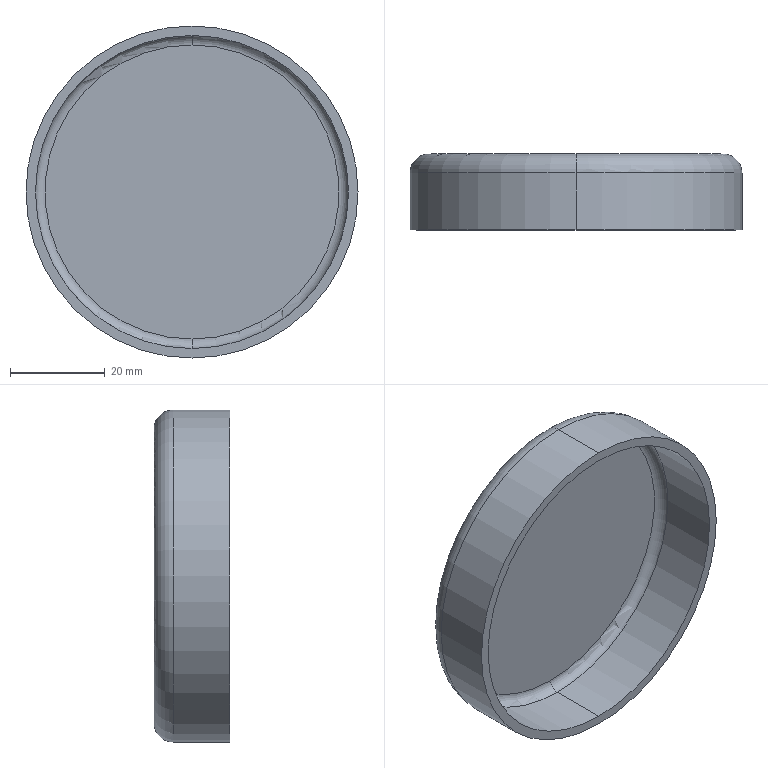Part | STEP file | 1 solid | 11 faces | box 70 x 16 x 70 mm | volume 11959 mm3 | torus 4 | cylinder 4 | plane 3 | commonest cylinder face diameters 66 x2 70 x2